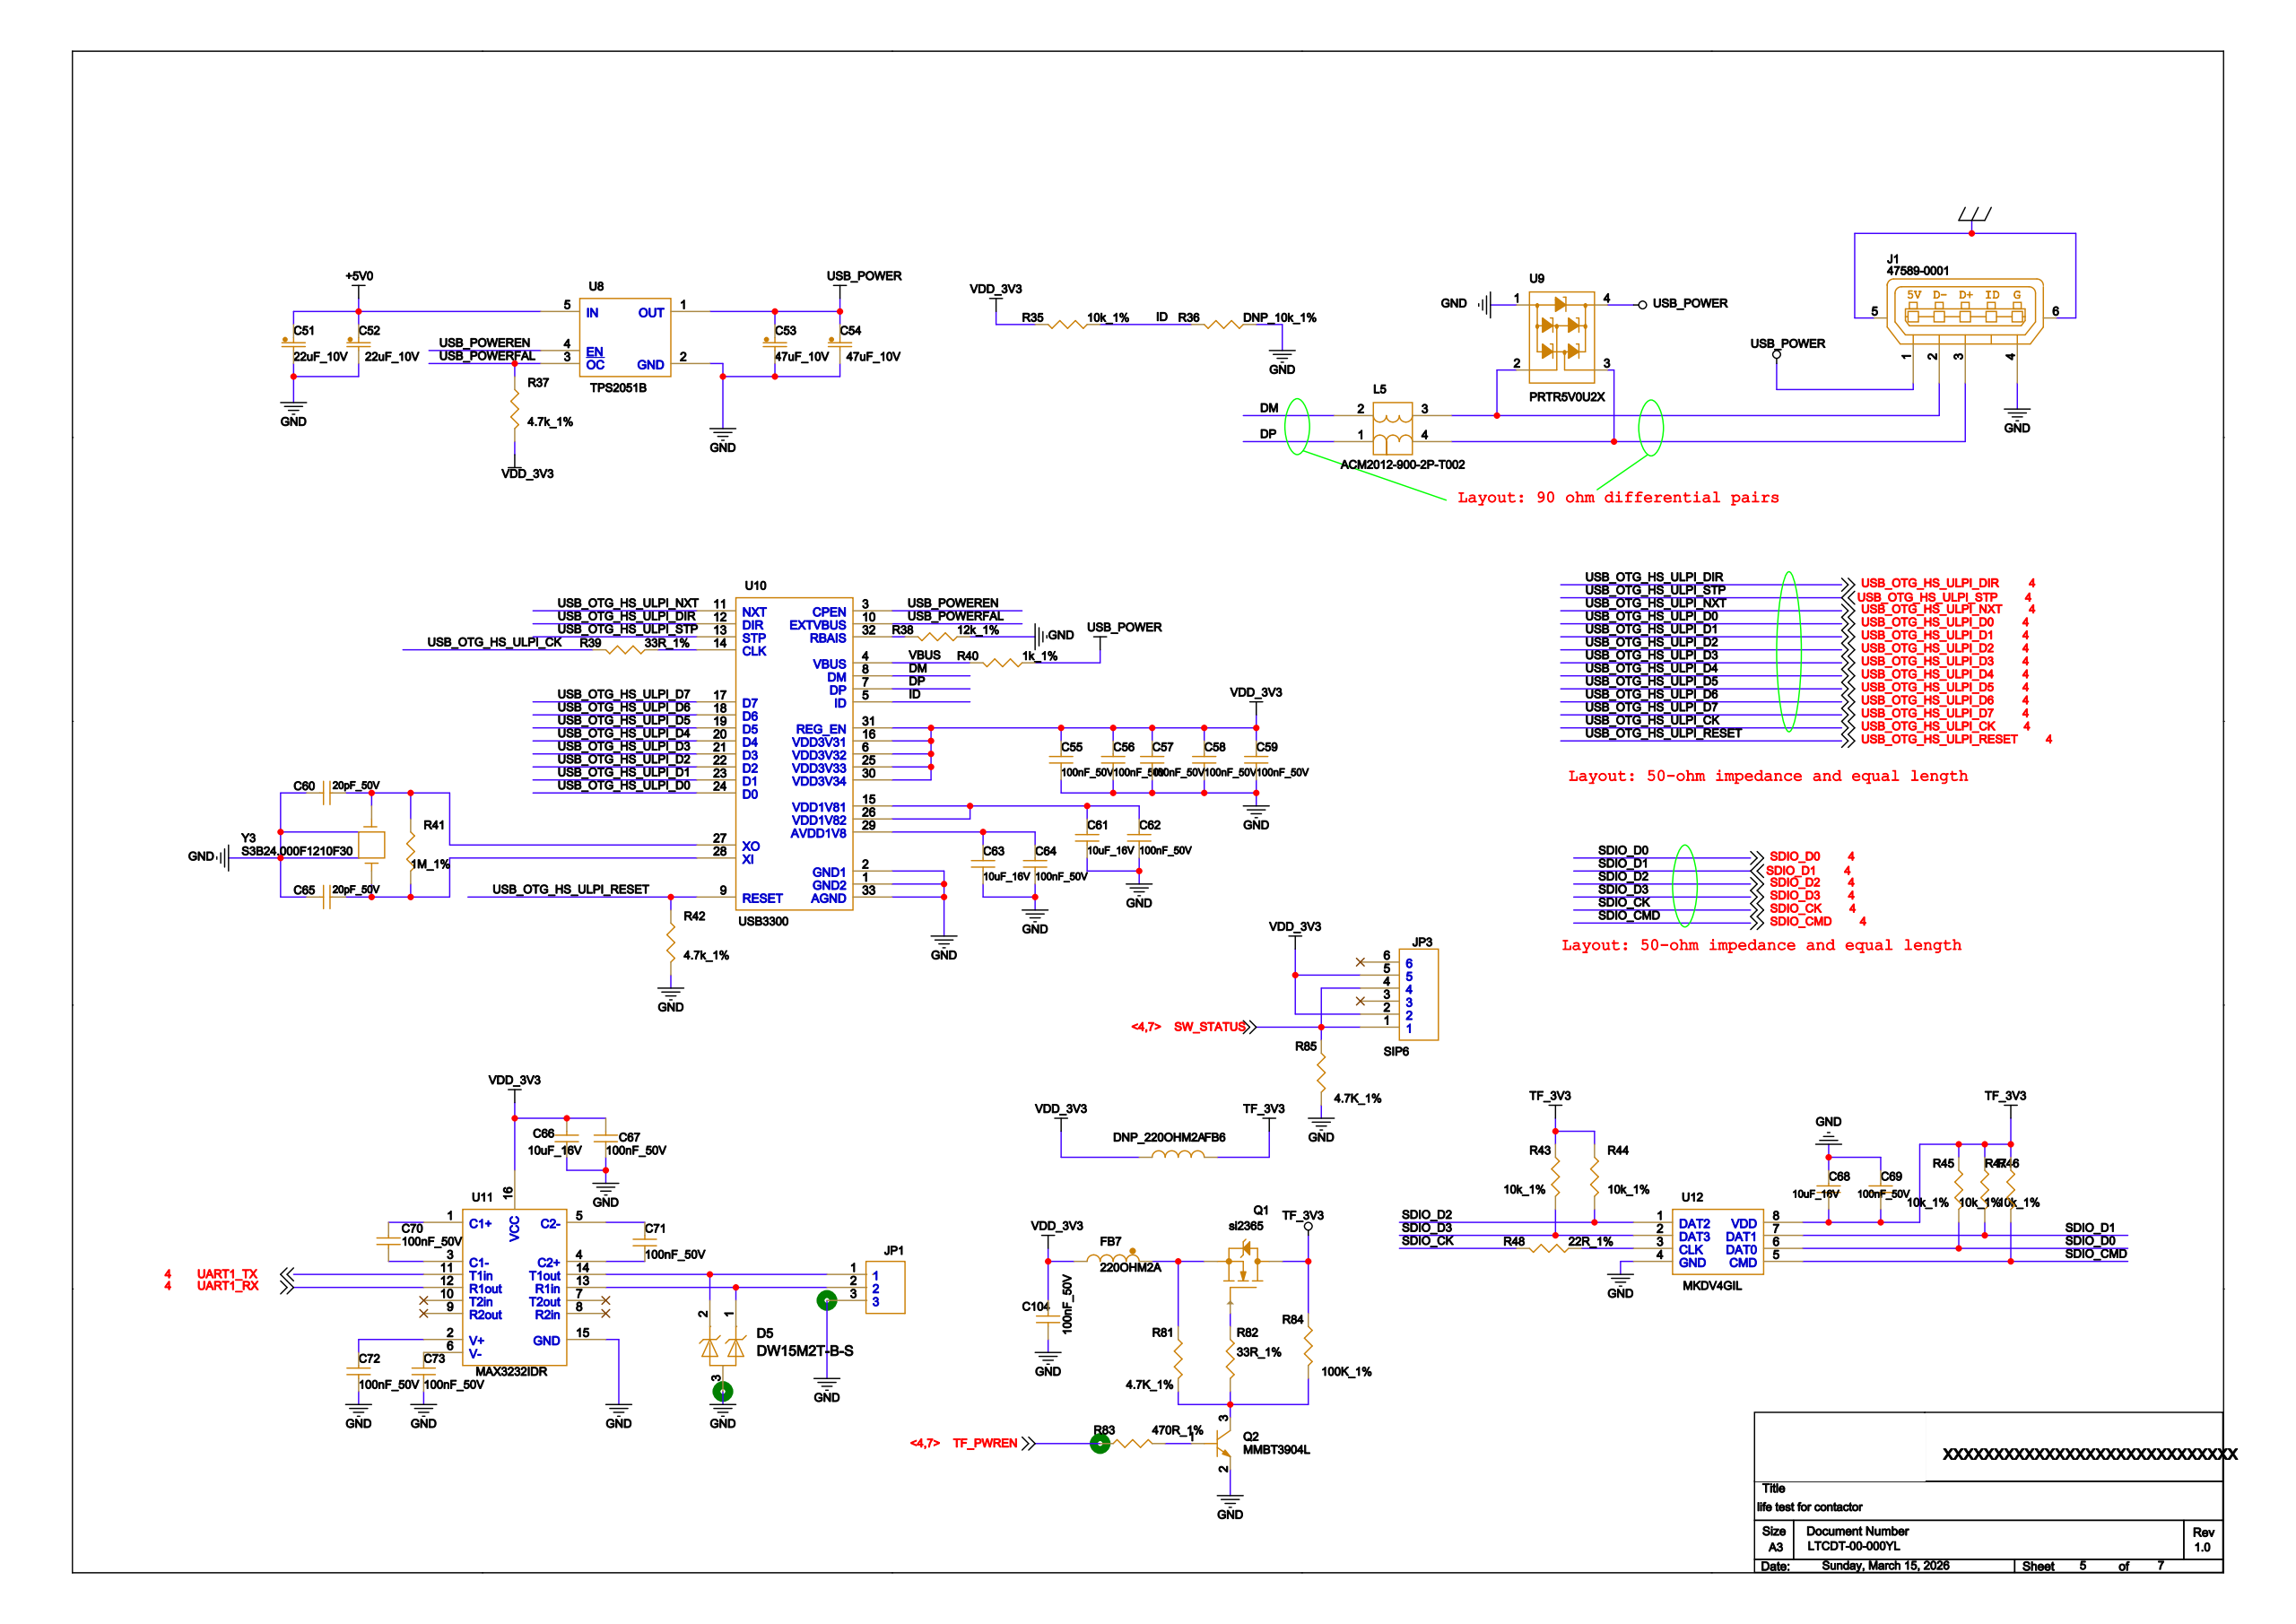Circuit board | Cadence Allegro | 260 parts | 211 nets | one sheet of the schematic
Parts on this sheet (reference | value | footprint):
C51 | 0805-C
C52 | 0805-C
C53 | 1206-C
C54 | 1206-C
C55 | 0603-C
C56 | 0603-C
C57 | 0603-C
C58 | 0603-C
C59 | 0603-C
C60 | 0603-C
C61 | 0603-C
C62 | 0603-C
C63 | 0603-C
C64 | 0603-C
C65 | 0603-C
C66 | 0603-C
C67 | 0603-C
C68 | 0603-C
C69 | 0603-C
C70 | 0603-C
C71 | 0603-C
C72 | 0603-C
C73 | 0603-C
C104 | 0603-C
D4 | SOD-123
D5 | SOT23-3-0_95-H1_11
FB7 | 0603-L
J1 | USB-A-TH_USB-231-ARY
JP1 | SIP3-2_54-MTP125
JP3 | 6MD1S202M2QES
L5 | L4-2_0X1_2X1_3-ACM2012
Q1 | SOT23-3-0_95-H1_11
Q2 | SOT23-3-0_95-H1_11
R35 | 0603-R
R36 | 0603-R
R37 | 0603-R
R38 | 0603-R
R39 | 0603-R
R40 | 0603-R
R41 | 0603-R
R42 | 0603-R
R43 | 0603-R
R44 | 0603-R
R45 | 0603-R
R46 | 0603-R
R47 | 0603-R
R48 | 0603-R
R81 | 0603-R
R82 | 0603-R
R83 | 0603-R
R84 | 0603-R
R85 | 0603-R
U8 | SOT-23-5-0_95-H1_45
U9 | SOT143-4-3_0X1_4-H1_15
U10 | QFN-32_L5_0-W5_0-P0_50-BL-EP3_4
U11 | SOIC16-1_27-5_4
U12 | LGA-8_L8_0-W6_0-TL_MKDV4GIL-AS
Y3 | X4-5_0X3_2-SG5032
Nets of these parts (net: part-pin ...):
GND: C51-2 C52-2 C53-2 C54-2 C55-2 C56-2 C57-2 C58-2 C59-2 C60-2 C61-2 C62-2 C63-2 C64-2 C65-2 C66-1 C67-1 C68-1 C69-1 C72-2 C73-2 C104-2 D5-3 J1-4 JP1-3 Q2-2 R36-2 R38-2 R42-1 R85-1 U8-2 U9-1 U11-15 U12-4 Y3-2 Y3-4 U10-1 U10-2 U10-33
N17321929: Q2-1 R83-1
TF_PWREN: R83-2
VDD_3V3: C55-1 C56-1 C57-1 C58-1 C59-1 C66-2 C67-2 C104-1 D4-1 FB7-2 JP3-2 JP3-5 R35-1 R37-1 U11-16 U10-6 U10-16 U10-25 U10-30 U10-31
GND_EARTH: J1-5 J1-6
+5V0: C51-1 C52-1 U8-5
N17242186: C61-1 C62-1 U10-15 U10-26
N17242080: C63-1 C64-1 U10-29
TF_3V3: C68-2 C69-2 Q1-3 R43-2 R44-2 R45-2 R46-2 R47-2 R84-2 U12-8
N17274007: C70-1 U11-1
N17274032: C70-2 U11-3
N17274034: C71-1 U11-4
N17274009: C71-2 U11-5
N17274078: C72-1 U11-2
N172740037: C73-1 U11-6
USB_POWER: C53-1 C54-1 J1-1 R40-2 U8-1 U9-4
N17241609: C60-1 R41-2 Y3-3 U10-27
N17241612: C65-1 R41-1 Y3-1 U10-28
N17215836: D4-2
N17274058: D5-1 JP1-2 U11-13
N17274050: D5-2 JP1-1 U11-14
N17321823: FB7-1 Q1-2 R81-2
N17246944: J1-2 L5-3 U9-2
N17246946: J1-3 L5-4 U9-3
SW_STATUS: JP3-1 JP3-4 R85-2
DP: L5-1 U10-7
DM: L5-2 U10-8
N17322467: Q1-1 R82-2
N17321892: Q2-3 R81-1 R82-1 R84-1
ID: R35-2 R36-1 U10-5
SDIO_D3: R43-1 U12-2
SDIO_D2: R44-1 U12-1
SDIO_D0: R45-1 U12-6
SDIO_D1: R46-1 U12-7
SDIO_CMD: R47-1 U12-5
USB_POWERFAL: R37-2 U8-3 U10-10
USB_OTG_HS_ULPI_RESET: R42-2 U10-9
N17245747: R38-1 U10-32
USB_OTG_HS_ULPI_CK: R39-1
N17241251: R39-2 U10-14
VBUS: R40-1 U10-4
SDIO_CK: R48-1
N17249016: R48-2 U12-3
USB_POWEREN: U8-4 U10-3
USB_OTG_HS_ULPI_D0: U10-24
USB_OTG_HS_ULPI_D1: U10-23
USB_OTG_HS_ULPI_D2: U10-22
USB_OTG_HS_ULPI_D3: U10-21
USB_OTG_HS_ULPI_D4: U10-20
USB_OTG_HS_ULPI_D5: U10-19
USB_OTG_HS_ULPI_D6: U10-18
USB_OTG_HS_ULPI_D7: U10-17
USB_OTG_HS_ULPI_DIR: U10-12
USB_OTG_HS_ULPI_NXT: U10-11
USB_OTG_HS_ULPI_STP: U10-13
UART1_RX: U11-12
UART1_TX: U11-11